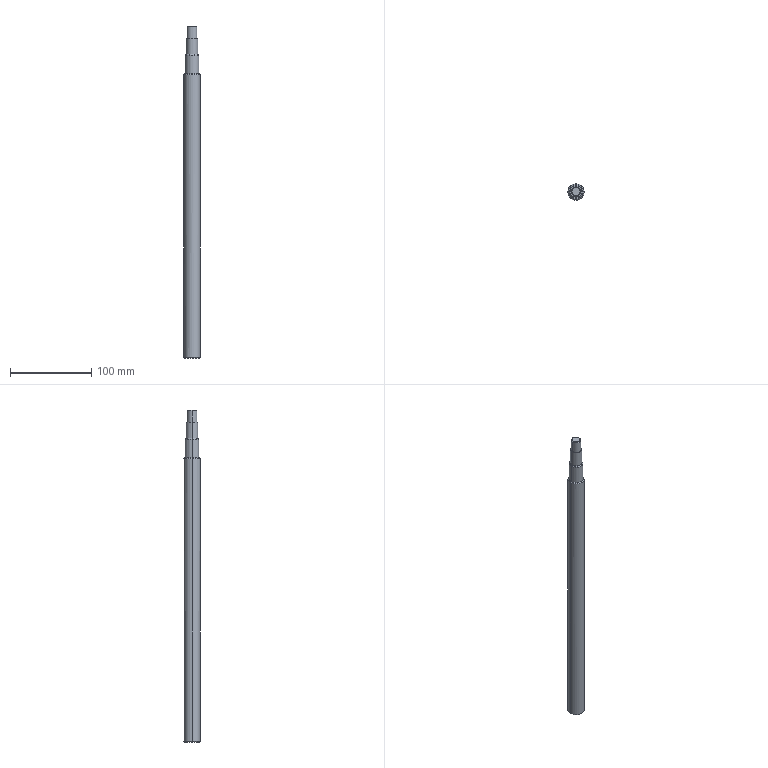Part | STEP file | fBY02F02M-00-27A | 1 solid | 21 faces | box 20 x 20 x 409 mm | volume 120074 mm3 | cylinder 8 | cone 8 | plane 5 | commonest cylinder face diameters 12 x2 14 x2 17 x2 20 x2
STEP:
#1=CARTESIAN_POINT('',(0.,0.,0.));
#2=DIRECTION('',(0.,0.,1.));
#3=DIRECTION('',(1.,0.,0.));
#4=AXIS2_PLACEMENT_3D('',#1,#2,#3);
#5=CARTESIAN_POINT('',(-10.,0.,349.));
#6=VERTEX_POINT('',#5);
#7=CARTESIAN_POINT('',(10.,0.,349.));
#8=VERTEX_POINT('',#7);
#9=CARTESIAN_POINT('',(0.,0.,349.));
#10=DIRECTION('',(0.,0.,-1.));
#11=DIRECTION('',(-1.,0.,0.));
#12=AXIS2_PLACEMENT_3D('',#9,#10,#11);
#13=CIRCLE('',#12,10.);
#14=CARTESIAN_POINT('',(0.,0.,350.));
#15=DIRECTION('',(0.,0.,-1.));
#16=DIRECTION('',(-1.,0.,0.));
#17=AXIS2_PLACEMENT_3D('',#14,#15,#16);
#18=CYLINDRICAL_SURFACE('',#17,10.);
#19=CARTESIAN_POINT('',(0.,1.));
#20=DIRECTION('',(1.,0.));
#21=VECTOR('',#20,1.);
#22=LINE('',#19,#21);
#23=(GEOMETRIC_REPRESENTATION_CONTEXT(2)PARAMETRIC_REPRESENTATION_CONTEXT()REPRESENTATION_CONTEXT('',''));
#24=DEFINITIONAL_REPRESENTATION('',(#22),#23);
#25=PCURVE('',#18,#24);
#26=CARTESIAN_POINT('',(0.,0.,349.));
#27=DIRECTION('',(0.,0.,-1.));
#28=DIRECTION('',(-1.,0.,0.));
#29=AXIS2_PLACEMENT_3D('',#26,#27,#28);
#30=CONICAL_SURFACE('',#29,10.,0.7854);
#31=CARTESIAN_POINT('',(0.,0.));
#32=DIRECTION('',(1.,0.));
#33=VECTOR('',#32,1.);
#34=LINE('',#31,#33);
#35=(GEOMETRIC_REPRESENTATION_CONTEXT(2)PARAMETRIC_REPRESENTATION_CONTEXT()REPRESENTATION_CONTEXT('',''));
#36=DEFINITIONAL_REPRESENTATION('',(#34),#35);
#37=PCURVE('',#30,#36);
#38=SURFACE_CURVE('',#13,(#25,#37),.PCURVE_S1.);
#39=EDGE_CURVE('',#6,#8,#38,.T.);
#40=ORIENTED_EDGE('',*,*,#39,.T.);
#41=CARTESIAN_POINT('',(10.,0.,1.));
#42=VERTEX_POINT('',#41);
#43=CARTESIAN_POINT('',(10.,0.,350.));
#44=DIRECTION('',(0.,0.,-1.));
#45=VECTOR('',#44,1.);
#46=LINE('',#43,#45);
#47=CARTESIAN_POINT('',(3.142,0.));
#48=DIRECTION('',(0.,1.));
#49=VECTOR('',#48,1.);
#50=LINE('',#47,#49);
#51=(GEOMETRIC_REPRESENTATION_CONTEXT(2)PARAMETRIC_REPRESENTATION_CONTEXT()REPRESENTATION_CONTEXT('',''));
#52=DEFINITIONAL_REPRESENTATION('',(#50),#51);
#53=PCURVE('',#18,#52);
#54=CARTESIAN_POINT('',(0.,0.,350.));
#55=DIRECTION('',(0.,0.,-1.));
#56=DIRECTION('',(-1.,0.,0.));
#57=AXIS2_PLACEMENT_3D('',#54,#55,#56);
#58=CYLINDRICAL_SURFACE('',#57,10.);
#59=CARTESIAN_POINT('',(3.142,0.));
#60=DIRECTION('',(0.,1.));
#61=VECTOR('',#60,1.);
#62=LINE('',#59,#61);
#63=(GEOMETRIC_REPRESENTATION_CONTEXT(2)PARAMETRIC_REPRESENTATION_CONTEXT()REPRESENTATION_CONTEXT('',''));
#64=DEFINITIONAL_REPRESENTATION('',(#62),#63);
#65=PCURVE('',#58,#64);
#66=SURFACE_CURVE('',#46,(#53,#65),.PCURVE_S1.);
#67=EDGE_CURVE('',#8,#42,#66,.T.);
#68=ORIENTED_EDGE('',*,*,#67,.T.);
#69=CARTESIAN_POINT('',(0.,10.,1.));
#70=VERTEX_POINT('',#69);
#71=CARTESIAN_POINT('',(0.,0.,1.));
#72=DIRECTION('',(0.,0.,1.));
#73=DIRECTION('',(-1.,0.,0.));
#74=AXIS2_PLACEMENT_3D('',#71,#72,#73);
#75=CIRCLE('',#74,10.);
#76=CARTESIAN_POINT('',(6.283,349.));
#77=DIRECTION('',(-1.,0.));
#78=VECTOR('',#77,1.);
#79=LINE('',#76,#78);
#80=(GEOMETRIC_REPRESENTATION_CONTEXT(2)PARAMETRIC_REPRESENTATION_CONTEXT()REPRESENTATION_CONTEXT('',''));
#81=DEFINITIONAL_REPRESENTATION('',(#79),#80);
#82=PCURVE('',#18,#81);
#83=CARTESIAN_POINT('',(0.,0.,1.));
#84=DIRECTION('',(0.,0.,1.));
#85=DIRECTION('',(0.,-1.,0.));
#86=AXIS2_PLACEMENT_3D('',#83,#84,#85);
#87=CONICAL_SURFACE('',#86,10.,0.7854);
#88=CARTESIAN_POINT('',(-1.571,0.));
#89=DIRECTION('',(1.,0.));
#90=VECTOR('',#89,1.);
#91=LINE('',#88,#90);
#92=(GEOMETRIC_REPRESENTATION_CONTEXT(2)PARAMETRIC_REPRESENTATION_CONTEXT()REPRESENTATION_CONTEXT('',''));
#93=DEFINITIONAL_REPRESENTATION('',(#91),#92);
#94=PCURVE('',#87,#93);
#95=SURFACE_CURVE('',#75,(#82,#94),.PCURVE_S1.);
#96=EDGE_CURVE('',#42,#70,#95,.T.);
#97=ORIENTED_EDGE('',*,*,#96,.T.);
#98=CARTESIAN_POINT('',(-10.,0.,1.));
#99=VERTEX_POINT('',#98);
#100=CARTESIAN_POINT('',(0.,0.,1.));
#101=DIRECTION('',(0.,0.,1.));
#102=DIRECTION('',(-1.,0.,0.));
#103=AXIS2_PLACEMENT_3D('',#100,#101,#102);
#104=CIRCLE('',#103,10.);
#105=CARTESIAN_POINT('',(6.283,349.));
#106=DIRECTION('',(-1.,0.));
#107=VECTOR('',#106,1.);
#108=LINE('',#105,#107);
#109=(GEOMETRIC_REPRESENTATION_CONTEXT(2)PARAMETRIC_REPRESENTATION_CONTEXT()REPRESENTATION_CONTEXT('',''));
#110=DEFINITIONAL_REPRESENTATION('',(#108),#109);
#111=PCURVE('',#18,#110);
#112=CARTESIAN_POINT('',(0.,0.,1.));
#113=DIRECTION('',(0.,0.,1.));
#114=DIRECTION('',(0.,-1.,0.));
#115=AXIS2_PLACEMENT_3D('',#112,#113,#114);
#116=CONICAL_SURFACE('',#115,10.,0.7854);
#117=CARTESIAN_POINT('',(-1.571,0.));
#118=DIRECTION('',(1.,0.));
#119=VECTOR('',#118,1.);
#120=LINE('',#117,#119);
#121=(GEOMETRIC_REPRESENTATION_CONTEXT(2)PARAMETRIC_REPRESENTATION_CONTEXT()REPRESENTATION_CONTEXT('',''));
#122=DEFINITIONAL_REPRESENTATION('',(#120),#121);
#123=PCURVE('',#116,#122);
#124=SURFACE_CURVE('',#104,(#111,#123),.PCURVE_S1.);
#125=EDGE_CURVE('',#70,#99,#124,.T.);
#126=ORIENTED_EDGE('',*,*,#125,.T.);
#127=CARTESIAN_POINT('',(-10.,0.,350.));
#128=DIRECTION('',(0.,0.,-1.));
#129=VECTOR('',#128,1.);
#130=LINE('',#127,#129);
#131=CARTESIAN_POINT('',(0.,0.));
#132=DIRECTION('',(0.,1.));
#133=VECTOR('',#132,1.);
#134=LINE('',#131,#133);
#135=(GEOMETRIC_REPRESENTATION_CONTEXT(2)PARAMETRIC_REPRESENTATION_CONTEXT()REPRESENTATION_CONTEXT('',''));
#136=DEFINITIONAL_REPRESENTATION('',(#134),#135);
#137=PCURVE('',#18,#136);
#138=CARTESIAN_POINT('',(6.283,0.));
#139=DIRECTION('',(0.,1.));
#140=VECTOR('',#139,1.);
#141=LINE('',#138,#140);
#142=(GEOMETRIC_REPRESENTATION_CONTEXT(2)PARAMETRIC_REPRESENTATION_CONTEXT()REPRESENTATION_CONTEXT('',''));
#143=DEFINITIONAL_REPRESENTATION('',(#141),#142);
#144=PCURVE('',#58,#143);
#145=SURFACE_CURVE('',#130,(#137,#144),.PCURVE_S1.);
#146=EDGE_CURVE('',#6,#99,#145,.T.);
#147=ORIENTED_EDGE('',*,*,#146,.F.);
#148=EDGE_LOOP('',(#40,#68,#97,#126,#147));
#149=FACE_BOUND('',#148,.T.);
#150=ADVANCED_FACE('',(#149),#18,.T.);
#151=CARTESIAN_POINT('',(0.,-9.,0.));
#152=VERTEX_POINT('',#151);
#153=CARTESIAN_POINT('',(0.,9.,0.));
#154=VERTEX_POINT('',#153);
#155=CARTESIAN_POINT('',(0.,0.,0.));
#156=DIRECTION('',(0.,0.,1.));
#157=DIRECTION('',(0.,-1.,0.));
#158=AXIS2_PLACEMENT_3D('',#155,#156,#157);
#159=CIRCLE('',#158,9.);
#160=CARTESIAN_POINT('',(0.,-1.));
#161=DIRECTION('',(1.,0.));
#162=VECTOR('',#161,1.);
#163=LINE('',#160,#162);
#164=(GEOMETRIC_REPRESENTATION_CONTEXT(2)PARAMETRIC_REPRESENTATION_CONTEXT()REPRESENTATION_CONTEXT('',''));
#165=DEFINITIONAL_REPRESENTATION('',(#163),#164);
#166=PCURVE('',#87,#165);
#167=CARTESIAN_POINT('',(0.,0.,0.));
#168=DIRECTION('',(0.,0.,1.));
#169=DIRECTION('',(1.,0.,0.));
#170=AXIS2_PLACEMENT_3D('',#167,#168,#169);
#171=PLANE('',#170);
#172=CARTESIAN_POINT('',(0.,0.));
#173=DIRECTION('',(0.,-1.));
#174=AXIS2_PLACEMENT_2D('',#172,#173);
#175=CIRCLE('',#174,9.);
#176=(GEOMETRIC_REPRESENTATION_CONTEXT(2)PARAMETRIC_REPRESENTATION_CONTEXT()REPRESENTATION_CONTEXT('',''));
#177=DEFINITIONAL_REPRESENTATION('',(#175),#176);
#178=PCURVE('',#171,#177);
#179=SURFACE_CURVE('',#159,(#166,#178),.PCURVE_S1.);
#180=EDGE_CURVE('',#152,#154,#179,.T.);
#181=ORIENTED_EDGE('',*,*,#180,.T.);
#182=CARTESIAN_POINT('',(0.,10.,1.));
#183=DIRECTION('',(0.,0.7071,0.7071));
#184=VECTOR('',#183,1.);
#185=LINE('',#182,#184);
#186=CARTESIAN_POINT('',(3.142,0.));
#187=DIRECTION('',(0.,1.));
#188=VECTOR('',#187,1.);
#189=LINE('',#186,#188);
#190=(GEOMETRIC_REPRESENTATION_CONTEXT(2)PARAMETRIC_REPRESENTATION_CONTEXT()REPRESENTATION_CONTEXT('',''));
#191=DEFINITIONAL_REPRESENTATION('',(#189),#190);
#192=PCURVE('',#87,#191);
#193=CARTESIAN_POINT('',(3.142,0.));
#194=DIRECTION('',(0.,1.));
#195=VECTOR('',#194,1.);
#196=LINE('',#193,#195);
#197=(GEOMETRIC_REPRESENTATION_CONTEXT(2)PARAMETRIC_REPRESENTATION_CONTEXT()REPRESENTATION_CONTEXT('',''));
#198=DEFINITIONAL_REPRESENTATION('',(#196),#197);
#199=PCURVE('',#116,#198);
#200=SURFACE_CURVE('',#185,(#192,#199),.PCURVE_S1.);
#201=EDGE_CURVE('',#154,#70,#200,.T.);
#202=ORIENTED_EDGE('',*,*,#201,.T.);
#203=ORIENTED_EDGE('',*,*,#96,.F.);
#204=CARTESIAN_POINT('',(0.,-10.,1.));
#205=VERTEX_POINT('',#204);
#206=CARTESIAN_POINT('',(0.,0.,1.));
#207=DIRECTION('',(0.,0.,1.));
#208=DIRECTION('',(-1.,0.,0.));
#209=AXIS2_PLACEMENT_3D('',#206,#207,#208);
#210=CIRCLE('',#209,10.);
#211=CARTESIAN_POINT('',(-1.571,0.));
#212=DIRECTION('',(1.,0.));
#213=VECTOR('',#212,1.);
#214=LINE('',#211,#213);
#215=(GEOMETRIC_REPRESENTATION_CONTEXT(2)PARAMETRIC_REPRESENTATION_CONTEXT()REPRESENTATION_CONTEXT('',''));
#216=DEFINITIONAL_REPRESENTATION('',(#214),#215);
#217=PCURVE('',#87,#216);
#218=CARTESIAN_POINT('',(6.283,349.));
#219=DIRECTION('',(-1.,0.));
#220=VECTOR('',#219,1.);
#221=LINE('',#218,#220);
#222=(GEOMETRIC_REPRESENTATION_CONTEXT(2)PARAMETRIC_REPRESENTATION_CONTEXT()REPRESENTATION_CONTEXT('',''));
#223=DEFINITIONAL_REPRESENTATION('',(#221),#222);
#224=PCURVE('',#58,#223);
#225=SURFACE_CURVE('',#210,(#217,#224),.PCURVE_S1.);
#226=EDGE_CURVE('',#205,#42,#225,.T.);
#227=ORIENTED_EDGE('',*,*,#226,.F.);
#228=CARTESIAN_POINT('',(0.,-10.,1.));
#229=DIRECTION('',(0.,-0.7071,0.7071));
#230=VECTOR('',#229,1.);
#231=LINE('',#228,#230);
#232=CARTESIAN_POINT('',(0.,0.));
#233=DIRECTION('',(0.,1.));
#234=VECTOR('',#233,1.);
#235=LINE('',#232,#234);
#236=(GEOMETRIC_REPRESENTATION_CONTEXT(2)PARAMETRIC_REPRESENTATION_CONTEXT()REPRESENTATION_CONTEXT('',''));
#237=DEFINITIONAL_REPRESENTATION('',(#235),#236);
#238=PCURVE('',#87,#237);
#239=CARTESIAN_POINT('',(6.283,0.));
#240=DIRECTION('',(0.,1.));
#241=VECTOR('',#240,1.);
#242=LINE('',#239,#241);
#243=(GEOMETRIC_REPRESENTATION_CONTEXT(2)PARAMETRIC_REPRESENTATION_CONTEXT()REPRESENTATION_CONTEXT('',''));
#244=DEFINITIONAL_REPRESENTATION('',(#242),#243);
#245=PCURVE('',#116,#244);
#246=SURFACE_CURVE('',#231,(#238,#245),.PCURVE_S1.);
#247=EDGE_CURVE('',#152,#205,#246,.T.);
#248=ORIENTED_EDGE('',*,*,#247,.F.);
#249=EDGE_LOOP('',(#181,#202,#203,#227,#248));
#250=FACE_BOUND('',#249,.T.);
#251=ADVANCED_FACE('',(#250),#87,.T.);
#252=CARTESIAN_POINT('',(-9.,0.,350.));
#253=VERTEX_POINT('',#252);
#254=CARTESIAN_POINT('',(9.,0.,350.));
#255=VERTEX_POINT('',#254);
#256=CARTESIAN_POINT('',(0.,0.,350.));
#257=DIRECTION('',(0.,0.,-1.));
#258=DIRECTION('',(-1.,0.,0.));
#259=AXIS2_PLACEMENT_3D('',#256,#257,#258);
#260=CIRCLE('',#259,9.);
#261=CARTESIAN_POINT('',(0.,-1.));
#262=DIRECTION('',(1.,0.));
#263=VECTOR('',#262,1.);
#264=LINE('',#261,#263);
#265=(GEOMETRIC_REPRESENTATION_CONTEXT(2)PARAMETRIC_REPRESENTATION_CONTEXT()REPRESENTATION_CONTEXT('',''));
#266=DEFINITIONAL_REPRESENTATION('',(#264),#265);
#267=PCURVE('',#30,#266);
#268=CARTESIAN_POINT('',(0.,0.,350.));
#269=DIRECTION('',(0.,0.,1.));
#270=DIRECTION('',(1.,0.,0.));
#271=AXIS2_PLACEMENT_3D('',#268,#269,#270);
#272=PLANE('',#271);
#273=CARTESIAN_POINT('',(-9.,0.));
#274=CARTESIAN_POINT('',(-9.,15.588));
#275=CARTESIAN_POINT('',(4.5,7.794));
#276=CARTESIAN_POINT('',(18.,0.));
#277=CARTESIAN_POINT('',(4.5,-7.794));
#278=CARTESIAN_POINT('',(-9.,-15.588));
#279=CARTESIAN_POINT('',(-9.,0.));
#280=(BOUNDED_CURVE()B_SPLINE_CURVE(2,(#273,#274,#275,#276,#277,#278,#279),.UNSPECIFIED.,.T.,.F.)B_SPLINE_CURVE_WITH_KNOTS((1,2,2,2,2,1),(-2.094,0.,2.094,4.189,6.283,8.378),.UNSPECIFIED.)CURVE()GEOMETRIC_REPRESENTATION_ITEM()RATIONAL_B_SPLINE_CURVE((1.,0.5,1.,0.5,1.,0.5,1.))REPRESENTATION_ITEM(''));
#281=(GEOMETRIC_REPRESENTATION_CONTEXT(2)PARAMETRIC_REPRESENTATION_CONTEXT()REPRESENTATION_CONTEXT('',''));
#282=DEFINITIONAL_REPRESENTATION('',(#280),#281);
#283=PCURVE('',#272,#282);
#284=SURFACE_CURVE('',#260,(#267,#283),.PCURVE_S1.);
#285=EDGE_CURVE('',#253,#255,#284,.T.);
#286=ORIENTED_EDGE('',*,*,#285,.T.);
#287=CARTESIAN_POINT('',(10.,0.,349.));
#288=DIRECTION('',(0.7071,0.,-0.7071));
#289=VECTOR('',#288,1.);
#290=LINE('',#287,#289);
#291=CARTESIAN_POINT('',(3.142,0.));
#292=DIRECTION('',(0.,1.));
#293=VECTOR('',#292,1.);
#294=LINE('',#291,#293);
#295=(GEOMETRIC_REPRESENTATION_CONTEXT(2)PARAMETRIC_REPRESENTATION_CONTEXT()REPRESENTATION_CONTEXT('',''));
#296=DEFINITIONAL_REPRESENTATION('',(#294),#295);
#297=PCURVE('',#30,#296);
#298=CARTESIAN_POINT('',(0.,0.,349.));
#299=DIRECTION('',(0.,0.,-1.));
#300=DIRECTION('',(-1.,0.,0.));
#301=AXIS2_PLACEMENT_3D('',#298,#299,#300);
#302=CONICAL_SURFACE('',#301,10.,0.7854);
#303=CARTESIAN_POINT('',(3.142,0.));
#304=DIRECTION('',(0.,1.));
#305=VECTOR('',#304,1.);
#306=LINE('',#303,#305);
#307=(GEOMETRIC_REPRESENTATION_CONTEXT(2)PARAMETRIC_REPRESENTATION_CONTEXT()REPRESENTATION_CONTEXT('',''));
#308=DEFINITIONAL_REPRESENTATION('',(#306),#307);
#309=PCURVE('',#302,#308);
#310=SURFACE_CURVE('',#290,(#297,#309),.PCURVE_S1.);
#311=EDGE_CURVE('',#255,#8,#310,.T.);
#312=ORIENTED_EDGE('',*,*,#311,.T.);
#313=ORIENTED_EDGE('',*,*,#39,.F.);
#314=CARTESIAN_POINT('',(-10.,0.,349.));
#315=DIRECTION('',(-0.7071,0.,-0.7071));
#316=VECTOR('',#315,1.);
#317=LINE('',#314,#316);
#318=CARTESIAN_POINT('',(0.,0.));
#319=DIRECTION('',(0.,1.));
#320=VECTOR('',#319,1.);
#321=LINE('',#318,#320);
#322=(GEOMETRIC_REPRESENTATION_CONTEXT(2)PARAMETRIC_REPRESENTATION_CONTEXT()REPRESENTATION_CONTEXT('',''));
#323=DEFINITIONAL_REPRESENTATION('',(#321),#322);
#324=PCURVE('',#30,#323);
#325=CARTESIAN_POINT('',(6.283,0.));
#326=DIRECTION('',(0.,1.));
#327=VECTOR('',#326,1.);
#328=LINE('',#325,#327);
#329=(GEOMETRIC_REPRESENTATION_CONTEXT(2)PARAMETRIC_REPRESENTATION_CONTEXT()REPRESENTATION_CONTEXT('',''));
#330=DEFINITIONAL_REPRESENTATION('',(#328),#329);
#331=PCURVE('',#302,#330);
#332=SURFACE_CURVE('',#317,(#324,#331),.PCURVE_S1.);
#333=EDGE_CURVE('',#253,#6,#332,.T.);
#334=ORIENTED_EDGE('',*,*,#333,.F.);
#335=EDGE_LOOP('',(#286,#312,#313,#334));
#336=FACE_BOUND('',#335,.T.);
#337=ADVANCED_FACE('',(#336),#30,.T.);
#338=CARTESIAN_POINT('',(-8.5,0.,373.));
#339=VERTEX_POINT('',#338);
#340=CARTESIAN_POINT('',(8.5,0.,373.));
#341=VERTEX_POINT('',#340);
#342=CARTESIAN_POINT('',(0.,0.,373.));
#343=DIRECTION('',(0.,0.,-1.));
#344=DIRECTION('',(-1.,0.,0.));
#345=AXIS2_PLACEMENT_3D('',#342,#343,#344);
#346=CIRCLE('',#345,8.5);
#347=CARTESIAN_POINT('',(0.,0.,374.));
#348=DIRECTION('',(0.,0.,-1.));
#349=DIRECTION('',(-1.,0.,0.));
#350=AXIS2_PLACEMENT_3D('',#347,#348,#349);
#351=CYLINDRICAL_SURFACE('',#350,8.5);
#352=CARTESIAN_POINT('',(0.,1.));
#353=DIRECTION('',(1.,0.));
#354=VECTOR('',#353,1.);
#355=LINE('',#352,#354);
#356=(GEOMETRIC_REPRESENTATION_CONTEXT(2)PARAMETRIC_REPRESENTATION_CONTEXT()REPRESENTATION_CONTEXT('',''));
#357=DEFINITIONAL_REPRESENTATION('',(#355),#356);
#358=PCURVE('',#351,#357);
#359=CARTESIAN_POINT('',(0.,0.,373.));
#360=DIRECTION('',(0.,0.,-1.));
#361=DIRECTION('',(-1.,0.,0.));
#362=AXIS2_PLACEMENT_3D('',#359,#360,#361);
#363=CONICAL_SURFACE('',#362,8.5,0.7854);
#364=CARTESIAN_POINT('',(0.,0.));
#365=DIRECTION('',(1.,0.));
#366=VECTOR('',#365,1.);
#367=LINE('',#364,#366);
#368=(GEOMETRIC_REPRESENTATION_CONTEXT(2)PARAMETRIC_REPRESENTATION_CONTEXT()REPRESENTATION_CONTEXT('',''));
#369=DEFINITIONAL_REPRESENTATION('',(#367),#368);
#370=PCURVE('',#363,#369);
#371=SURFACE_CURVE('',#346,(#358,#370),.PCURVE_S1.);
#372=EDGE_CURVE('',#339,#341,#371,.T.);
#373=ORIENTED_EDGE('',*,*,#372,.T.);
#374=CARTESIAN_POINT('',(8.5,0.,350.));
#375=VERTEX_POINT('',#374);
#376=CARTESIAN_POINT('',(8.5,0.,374.));
#377=DIRECTION('',(0.,0.,-1.));
#378=VECTOR('',#377,1.);
#379=LINE('',#376,#378);
#380=CARTESIAN_POINT('',(3.142,0.));
#381=DIRECTION('',(0.,1.));
#382=VECTOR('',#381,1.);
#383=LINE('',#380,#382);
#384=(GEOMETRIC_REPRESENTATION_CONTEXT(2)PARAMETRIC_REPRESENTATION_CONTEXT()REPRESENTATION_CONTEXT('',''));
#385=DEFINITIONAL_REPRESENTATION('',(#383),#384);
#386=PCURVE('',#351,#385);
#387=CARTESIAN_POINT('',(0.,0.,374.));
#388=DIRECTION('',(0.,0.,-1.));
#389=DIRECTION('',(-1.,0.,0.));
#390=AXIS2_PLACEMENT_3D('',#387,#388,#389);
#391=CYLINDRICAL_SURFACE('',#390,8.5);
#392=CARTESIAN_POINT('',(3.142,0.));
#393=DIRECTION('',(0.,1.));
#394=VECTOR('',#393,1.);
#395=LINE('',#392,#394);
#396=(GEOMETRIC_REPRESENTATION_CONTEXT(2)PARAMETRIC_REPRESENTATION_CONTEXT()REPRESENTATION_CONTEXT('',''));
#397=DEFINITIONAL_REPRESENTATION('',(#395),#396);
#398=PCURVE('',#391,#397);
#399=SURFACE_CURVE('',#379,(#386,#398),.PCURVE_S1.);
#400=EDGE_CURVE('',#341,#375,#399,.T.);
#401=ORIENTED_EDGE('',*,*,#400,.T.);
#402=CARTESIAN_POINT('',(-8.5,0.,350.));
#403=VERTEX_POINT('',#402);
#404=CARTESIAN_POINT('',(0.,0.,350.));
#405=DIRECTION('',(0.,0.,-1.));
#406=DIRECTION('',(-1.,0.,0.));
#407=AXIS2_PLACEMENT_3D('',#404,#405,#406);
#408=CIRCLE('',#407,8.5);
#409=CARTESIAN_POINT('',(0.,24.));
#410=DIRECTION('',(1.,0.));
#411=VECTOR('',#410,1.);
#412=LINE('',#409,#411);
#413=(GEOMETRIC_REPRESENTATION_CONTEXT(2)PARAMETRIC_REPRESENTATION_CONTEXT()REPRESENTATION_CONTEXT('',''));
#414=DEFINITIONAL_REPRESENTATION('',(#412),#413);
#415=PCURVE('',#351,#414);
#416=CARTESIAN_POINT('',(-8.5,0.));
#417=CARTESIAN_POINT('',(-8.5,14.722));
#418=CARTESIAN_POINT('',(4.25,7.361));
#419=CARTESIAN_POINT('',(17.,0.));
#420=CARTESIAN_POINT('',(4.25,-7.361));
#421=CARTESIAN_POINT('',(-8.5,-14.722));
#422=CARTESIAN_POINT('',(-8.5,0.));
#423=(BOUNDED_CURVE()B_SPLINE_CURVE(2,(#416,#417,#418,#419,#420,#421,#422),.UNSPECIFIED.,.T.,.F.)B_SPLINE_CURVE_WITH_KNOTS((1,2,2,2,2,1),(-2.094,0.,2.094,4.189,6.283,8.378),.UNSPECIFIED.)CURVE()GEOMETRIC_REPRESENTATION_ITEM()RATIONAL_B_SPLINE_CURVE((1.,0.5,1.,0.5,1.,0.5,1.))REPRESENTATION_ITEM(''));
#424=(GEOMETRIC_REPRESENTATION_CONTEXT(2)PARAMETRIC_REPRESENTATION_CONTEXT()REPRESENTATION_CONTEXT('',''));
#425=DEFINITIONAL_REPRESENTATION('',(#423),#424);
#426=PCURVE('',#272,#425);
#427=SURFACE_CURVE('',#408,(#415,#426),.PCURVE_S1.);
#428=EDGE_CURVE('',#403,#375,#427,.T.);
#429=ORIENTED_EDGE('',*,*,#428,.F.);
#430=CARTESIAN_POINT('',(-8.5,0.,374.));
#431=DIRECTION('',(0.,0.,-1.));
#432=VECTOR('',#431,1.);
#433=LINE('',#430,#432);
#434=CARTESIAN_POINT('',(0.,0.));
#435=DIRECTION('',(0.,1.));
#436=VECTOR('',#435,1.);
#437=LINE('',#434,#436);
#438=(GEOMETRIC_REPRESENTATION_CONTEXT(2)PARAMETRIC_REPRESENTATION_CONTEXT()REPRESENTATION_CONTEXT('',''));
#439=DEFINITIONAL_REPRESENTATION('',(#437),#438);
#440=PCURVE('',#351,#439);
#441=CARTESIAN_POINT('',(6.283,0.));
#442=DIRECTION('',(0.,1.));
#443=VECTOR('',#442,1.);
#444=LINE('',#441,#443);
#445=(GEOMETRIC_REPRESENTATION_CONTEXT(2)PARAMETRIC_REPRESENTATION_CONTEXT()REPRESENTATION_CONTEXT('',''));
#446=DEFINITIONAL_REPRESENTATION('',(#444),#445);
#447=PCURVE('',#391,#446);
#448=SURFACE_CURVE('',#433,(#440,#447),.PCURVE_S1.);
#449=EDGE_CURVE('',#339,#403,#448,.T.);
#450=ORIENTED_EDGE('',*,*,#449,.F.);
#451=EDGE_LOOP('',(#373,#401,#429,#450));
#452=FACE_BOUND('',#451,.T.);
#453=ADVANCED_FACE('',(#452),#351,.T.);
#454=CARTESIAN_POINT('',(-7.5,0.,374.));
#455=VERTEX_POINT('',#454);
#456=CARTESIAN_POINT('',(7.5,0.,374.));
#457=VERTEX_POINT('',#456);
#458=CARTESIAN_POINT('',(0.,0.,374.));
#459=DIRECTION('',(0.,0.,-1.));
#460=DIRECTION('',(-1.,0.,0.));
#461=AXIS2_PLACEMENT_3D('',#458,#459,#460);
#462=CIRCLE('',#461,7.5);
#463=CARTESIAN_POINT('',(0.,-1.));
#464=DIRECTION('',(1.,0.));
#465=VECTOR('',#464,1.);
#466=LINE('',#463,#465);
#467=(GEOMETRIC_REPRESENTATION_CONTEXT(2)PARAMETRIC_REPRESENTATION_CONTEXT()REPRESENTATION_CONTEXT('',''));
#468=DEFINITIONAL_REPRESENTATION('',(#466),#467);
#469=PCURVE('',#363,#468);
#470=CARTESIAN_POINT('',(0.,0.,374.));
#471=DIRECTION('',(0.,0.,1.));
#472=DIRECTION('',(1.,0.,0.));
#473=AXIS2_PLACEMENT_3D('',#470,#471,#472);
#474=PLANE('',#473);
#475=CARTESIAN_POINT('',(-7.5,0.));
#476=CARTESIAN_POINT('',(-7.5,12.99));
#477=CARTESIAN_POINT('',(3.75,6.495));
#478=CARTESIAN_POINT('',(15.,0.));
#479=CARTESIAN_POINT('',(3.75,-6.495));
#480=CARTESIAN_POINT('',(-7.5,-12.99));
#481=CARTESIAN_POINT('',(-7.5,0.));
#482=(BOUNDED_CURVE()B_SPLINE_CURVE(2,(#475,#476,#477,#478,#479,#480,#481),.UNSPECIFIED.,.T.,.F.)B_SPLINE_CURVE_WITH_KNOTS((1,2,2,2,2,1),(-2.094,0.,2.094,4.189,6.283,8.378),.UNSPECIFIED.)CURVE()GEOMETRIC_REPRESENTATION_ITEM()RATIONAL_B_SPLINE_CURVE((1.,0.5,1.,0.5,1.,0.5,1.))REPRESENTATION_ITEM(''));
#483=(GEOMETRIC_REPRESENTATION_CONTEXT(2)PARAMETRIC_REPRESENTATION_CONTEXT()REPRESENTATION_CONTEXT('',''));
#484=DEFINITIONAL_REPRESENTATION('',(#482),#483);
#485=PCURVE('',#474,#484);
#486=SURFACE_CURVE('',#462,(#469,#485),.PCURVE_S1.);
#487=EDGE_CURVE('',#455,#457,#486,.T.);
#488=ORIENTED_EDGE('',*,*,#487,.T.);
#489=CARTESIAN_POINT('',(8.5,0.,373.));
#490=DIRECTION('',(0.7071,0.,-0.7071));
#491=VECTOR('',#490,1.);
#492=LINE('',#489,#491);
#493=CARTESIAN_POINT('',(3.142,0.));
#494=DIRECTION('',(0.,1.));
#495=VECTOR('',#494,1.);
#496=LINE('',#493,#495);
#497=(GEOMETRIC_REPRESENTATION_CONTEXT(2)PARAMETRIC_REPRESENTATION_CONTEXT()REPRESENTATION_CONTEXT('',''));
#498=DEFINITIONAL_REPRESENTATION('',(#496),#497);
#499=PCURVE('',#363,#498);
#500=CARTESIAN_POINT('',(0.,0.,373.));
#501=DIRECTION('',(0.,0.,-1.));
#502=DIRECTION('',(-1.,0.,0.));
#503=AXIS2_PLACEMENT_3D('',#500,#501,#502);
#504=CONICAL_SURFACE('',#503,8.5,0.7854);
#505=CARTESIAN_POINT('',(3.142,0.));
#506=DIRECTION('',(0.,1.));
#507=VECTOR('',#506,1.);
#508=LINE('',#505,#507);
#509=(GEOMETRIC_REPRESENTATION_CONTEXT(2)PARAMETRIC_REPRESENTATION_CONTEXT()REPRESENTATION_CONTEXT('',''));
#510=DEFINITIONAL_REPRESENTATION('',(#508),#509);
#511=PCURVE('',#504,#510);
#512=SURFACE_CURVE('',#492,(#499,#511),.PCURVE_S1.);
#513=EDGE_CURVE('',#457,#341,#512,.T.);
#514=ORIENTED_EDGE('',*,*,#513,.T.);
#515=ORIENTED_EDGE('',*,*,#372,.F.);
#516=CARTESIAN_POINT('',(-8.5,0.,373.));
#517=DIRECTION('',(-0.7071,0.,-0.7071));
#518=VECTOR('',#517,1.);
#519=LINE('',#516,#518);
#520=CARTESIAN_POINT('',(0.,0.));
#521=DIRECTION('',(0.,1.));
#522=VECTOR('',#521,1.);
#523=LINE('',#520,#522);
#524=(GEOMETRIC_REPRESENTATION_CONTEXT(2)PARAMETRIC_REPRESENTATION_CONTEXT()REPRESENTATION_CONTEXT('',''));
#525=DEFINITIONAL_REPRESENTATION('',(#523),#524);
#526=PCURVE('',#363,#525);
#527=CARTESIAN_POINT('',(6.283,0.));
#528=DIRECTION('',(0.,1.));
#529=VECTOR('',#528,1.);
#530=LINE('',#527,#529);
#531=(GEOMETRIC_REPRESENTATION_CONTEXT(2)PARAMETRIC_REPRESENTATION_CONTEXT()REPRESENTATION_CONTEXT('',''));
#532=DEFINITIONAL_REPRESENTATION('',(#530),#531);
#533=PCURVE('',#504,#532);
#534=SURFACE_CURVE('',#519,(#526,#533),.PCURVE_S1.);
#535=EDGE_CURVE('',#455,#339,#534,.T.);
#536=ORIENTED_EDGE('',*,*,#535,.F.);
#537=EDGE_LOOP('',(#488,#514,#515,#536));
#538=FACE_BOUND('',#537,.T.);
#539=ADVANCED_FACE('',(#538),#363,.T.);
#540=CARTESIAN_POINT('',(-7.,0.,394.));
#541=VERTEX_POINT('',#540);
#542=CARTESIAN_POINT('',(7.,0.,394.));
#543=VERTEX_POINT('',#542);
#544=CARTESIAN_POINT('',(0.,0.,394.));
#545=DIRECTION('',(0.,0.,-1.));
#546=DIRECTION('',(-1.,0.,0.));
#547=AXIS2_PLACEMENT_3D('',#544,#545,#546);
#548=CIRCLE('',#547,7.);
#549=CARTESIAN_POINT('',(0.,0.,409.));
#550=DIRECTION('',(0.,0.,-1.));
#551=DIRECTION('',(-1.,0.,0.));
#552=AXIS2_PLACEMENT_3D('',#549,#550,#551);
#553=CYLINDRICAL_SURFACE('',#552,7.);
#554=CARTESIAN_POINT('',(0.,15.));
#555=DIRECTION('',(1.,0.));
#556=VECTOR('',#555,1.);
#557=LINE('',#554,#556);
#558=(GEOMETRIC_REPRESENTATION_CONTEXT(2)PARAMETRIC_REPRESENTATION_CONTEXT()REPRESENTATION_CONTEXT('',''));
#559=DEFINITIONAL_REPRESENTATION('',(#557),#558);
#560=PCURVE('',#553,#559);
#561=CARTESIAN_POINT('',(0.,0.,394.));
#562=DIRECTION('',(0.,0.,1.));
#563=DIRECTION('',(1.,0.,0.));
#564=AXIS2_PLACEMENT_3D('',#561,#562,#563);
#565=PLANE('',#564);
#566=CARTESIAN_POINT('',(-7.,0.));
#567=CARTESIAN_POINT('',(-7.,12.124));
#568=CARTESIAN_POINT('',(3.5,6.062));
#569=CARTESIAN_POINT('',(14.,0.));
#570=CARTESIAN_POINT('',(3.5,-6.062));
#571=CARTESIAN_POINT('',(-7.,-12.124));
#572=CARTESIAN_POINT('',(-7.,0.));
#573=(BOUNDED_CURVE()B_SPLINE_CURVE(2,(#566,#567,#568,#569,#570,#571,#572),.UNSPECIFIED.,.T.,.F.)B_SPLINE_CURVE_WITH_KNOTS((1,2,2,2,2,1),(-2.094,0.,2.094,4.189,6.283,8.378),.UNSPECIFIED.)CURVE()GEOMETRIC_REPRESENTATION_ITEM()RATIONAL_B_SPLINE_CURVE((1.,0.5,1.,0.5,1.,0.5,1.))REPRESENTATION_ITEM(''));
#574=(GEOMETRIC_REPRESENTATION_CONTEXT(2)PARAMETRIC_REPRESENTATION_CONTEXT()REPRESENTATION_CONTEXT('',''));
#575=DEFINITIONAL_REPRESENTATION('',(#573),#574);
#576=PCURVE('',#565,#575);
#577=SURFACE_CURVE('',#548,(#560,#576),.PCURVE_S1.);
#578=EDGE_CURVE('',#541,#543,#577,.T.);
#579=ORIENTED_EDGE('',*,*,#578,.T.);
#580=CARTESIAN_POINT('',(7.,0.,374.));
#581=VERTEX_POINT('',#580);
#582=CARTESIAN_POINT('',(7.,0.,409.));
#583=DIRECTION('',(0.,0.,-1.));
#584=VECTOR('',#583,1.);
#585=LINE('',#582,#584);
#586=CARTESIAN_POINT('',(3.142,0.));
#587=DIRECTION('',(0.,1.));
#588=VECTOR('',#587,1.);
#589=LINE('',#586,#588);
#590=(GEOMETRIC_REPRESENTATION_CONTEXT(2)PARAMETRIC_REPRESENTATION_CONTEXT()REPRESENTATION_CONTEXT('',''));
#591=DEFINITIONAL_REPRESENTATION('',(#589),#590);
#592=PCURVE('',#553,#591);
#593=CARTESIAN_POINT('',(0.,0.,409.));
#594=DIRECTION('',(0.,0.,-1.));
#595=DIRECTION('',(-1.,0.,0.));
#596=AXIS2_PLACEMENT_3D('',#593,#594,#595);
#597=CYLINDRICAL_SURFACE('',#596,7.);
#598=CARTESIAN_POINT('',(3.142,0.));
#599=DIRECTION('',(0.,1.));
#600=VECTOR('',#599,1.);
#601=LINE('',#598,#600);
#602=(GEOMETRIC_REPRESENTATION_CONTEXT(2)PARAMETRIC_REPRESENTATION_CONTEXT()REPRESENTATION_CONTEXT('',''));
#603=DEFINITIONAL_REPRESENTATION('',(#601),#602);
#604=PCURVE('',#597,#603);
#605=SURFACE_CURVE('',#585,(#592,#604),.PCURVE_S1.);
#606=EDGE_CURVE('',#543,#581,#605,.T.);
#607=ORIENTED_EDGE('',*,*,#606,.T.);
#608=CARTESIAN_POINT('',(-7.,0.,374.));
#609=VERTEX_POINT('',#608);
#610=CARTESIAN_POINT('',(0.,0.,374.));
#611=DIRECTION('',(0.,0.,-1.));
#612=DIRECTION('',(-1.,0.,0.));
#613=AXIS2_PLACEMENT_3D('',#610,#611,#612);
#614=CIRCLE('',#613,7.);
#615=CARTESIAN_POINT('',(0.,35.));
#616=DIRECTION('',(1.,0.));
#617=VECTOR('',#616,1.);
#618=LINE('',#615,#617);
#619=(GEOMETRIC_REPRESENTATION_CONTEXT(2)PARAMETRIC_REPRESENTATION_CONTEXT()REPRESENTATION_CONTEXT('',''));
#620=DEFINITIONAL_REPRESENTATION('',(#618),#619);
#621=PCURVE('',#553,#620);
#622=CARTESIAN_POINT('',(-7.,0.));
#623=CARTESIAN_POINT('',(-7.,12.124));
#624=CARTESIAN_POINT('',(3.5,6.062));
#625=CARTESIAN_POINT('',(14.,0.));
#626=CARTESIAN_POINT('',(3.5,-6.062));
#627=CARTESIAN_POINT('',(-7.,-12.124));
#628=CARTESIAN_POINT('',(-7.,0.));
#629=(BOUNDED_CURVE()B_SPLINE_CURVE(2,(#622,#623,#624,#625,#626,#627,#628),.UNSPECIFIED.,.T.,.F.)B_SPLINE_CURVE_WITH_KNOTS((1,2,2,2,2,1),(-2.094,0.,2.094,4.189,6.283,8.378),.UNSPECIFIED.)CURVE()GEOMETRIC_REPRESENTATION_ITEM()RATIONAL_B_SPLINE_CURVE((1.,0.5,1.,0.5,1.,0.5,1.))REPRESENTATION_ITEM(''));
#630=(GEOMETRIC_REPRESENTATION_CONTEXT(2)PARAMETRIC_REPRESENTATION_CONTEXT()REPRESENTATION_CONTEXT('',''));
#631=DEFINITIONAL_REPRESENTATION('',(#629),#630);
#632=PCURVE('',#474,#631);
#633=SURFACE_CURVE('',#614,(#621,#632),.PCURVE_S1.);
#634=EDGE_CURVE('',#609,#581,#633,.T.);
#635=ORIENTED_EDGE('',*,*,#634,.F.);
#636=CARTESIAN_POINT('',(-7.,0.,409.));
#637=DIRECTION('',(0.,0.,-1.));
#638=VECTOR('',#637,1.);
#639=LINE('',#636,#638);
#640=CARTESIAN_POINT('',(0.,0.));
#641=DIRECTION('',(0.,1.));
#642=VECTOR('',#641,1.);
#643=LINE('',#640,#642);
#644=(GEOMETRIC_REPRESENTATION_CONTEXT(2)PARAMETRIC_REPRESENTATION_CONTEXT()REPRESENTATION_CONTEXT('',''));
#645=DEFINITIONAL_REPRESENTATION('',(#643),#644);
#646=PCURVE('',#553,#645);
#647=CARTESIAN_POINT('',(6.283,0.));
#648=DIRECTION('',(0.,1.));
#649=VECTOR('',#648,1.);
#650=LINE('',#647,#649);
#651=(GEOMETRIC_REPRESENTATION_CONTEXT(2)PARAMETRIC_REPRESENTATION_CONTEXT()REPRESENTATION_CONTEXT('',''));
#652=DEFINITIONAL_REPRESENTATION('',(#650),#651);
#653=PCURVE('',#597,#652);
#654=SURFACE_CURVE('',#639,(#646,#653),.PCURVE_S1.);
#655=EDGE_CURVE('',#541,#609,#654,.T.);
#656=ORIENTED_EDGE('',*,*,#655,.F.);
#657=EDGE_LOOP('',(#579,#607,#635,#656));
#658=FACE_BOUND('',#657,.T.);
#659=ADVANCED_FACE('',(#658),#553,.T.);
#660=CARTESIAN_POINT('',(-6.,0.,394.));
#661=VERTEX_POINT('',#660);
#662=CARTESIAN_POINT('',(6.,0.,394.));
#663=VERTEX_POINT('',#662);
#664=CARTESIAN_POINT('',(0.,0.,394.));
#665=DIRECTION('',(0.,0.,-1.));
#666=DIRECTION('',(1.,0.,0.));
#667=AXIS2_PLACEMENT_3D('',#664,#665,#666);
#668=CIRCLE('',#667,6.);
#669=CARTESIAN_POINT('',(0.,0.,394.));
#670=DIRECTION('',(0.,0.,1.));
#671=DIRECTION('',(1.,0.,0.));
#672=AXIS2_PLACEMENT_3D('',#669,#670,#671);
#673=CYLINDRICAL_SURFACE('',#672,6.);
#674=CARTESIAN_POINT('',(6.283,0.));
#675=DIRECTION('',(-1.,0.));
#676=VECTOR('',#675,1.);
#677=LINE('',#674,#676);
#678=(GEOMETRIC_REPRESENTATION_CONTEXT(2)PARAMETRIC_REPRESENTATION_CONTEXT()REPRESENTATION_CONTEXT('',''));
#679=DEFINITIONAL_REPRESENTATION('',(#677),#678);
#680=PCURVE('',#673,#679);
#681=CARTESIAN_POINT('',(6.,0.));
#682=CARTESIAN_POINT('',(6.,-10.392));
#683=CARTESIAN_POINT('',(-3.,-5.196));
#684=CARTESIAN_POINT('',(-12.,0.));
#685=CARTESIAN_POINT('',(-3.,5.196));
#686=CARTESIAN_POINT('',(6.,10.392));
#687=CARTESIAN_POINT('',(6.,0.));
#688=(BOUNDED_CURVE()B_SPLINE_CURVE(2,(#681,#682,#683,#684,#685,#686,#687),.UNSPECIFIED.,.T.,.F.)B_SPLINE_CURVE_WITH_KNOTS((1,2,2,2,2,1),(-2.094,0.,2.094,4.189,6.283,8.378),.UNSPECIFIED.)CURVE()GEOMETRIC_REPRESENTATION_ITEM()RATIONAL_B_SPLINE_CURVE((1.,0.5,1.,0.5,1.,0.5,1.))REPRESENTATION_ITEM(''));
#689=(GEOMETRIC_REPRESENTATION_CONTEXT(2)PARAMETRIC_REPRESENTATION_CONTEXT()REPRESENTATION_CONTEXT('',''));
#690=DEFINITIONAL_REPRESENTATION('',(#688),#689);
#691=PCURVE('',#565,#690);
#692=SURFACE_CURVE('',#668,(#680,#691),.PCURVE_S1.);
#693=EDGE_CURVE('',#661,#663,#692,.T.);
#694=ORIENTED_EDGE('',*,*,#693,.F.);
#695=CARTESIAN_POINT('',(-6.,0.,408.));
#696=VERTEX_POINT('',#695);
#697=CARTESIAN_POINT('',(-6.,0.,394.));
#698=DIRECTION('',(0.,0.,1.));
#699=VECTOR('',#698,1.);
#700=LINE('',#697,#699);
#701=CARTESIAN_POINT('',(3.142,0.));
#702=DIRECTION('',(0.,1.));
#703=VECTOR('',#702,1.);
#704=LINE('',#701,#703);
#705=(GEOMETRIC_REPRESENTATION_CONTEXT(2)PARAMETRIC_REPRESENTATION_CONTEXT()REPRESENTATION_CONTEXT('',''));
#706=DEFINITIONAL_REPRESENTATION('',(#704),#705);
#707=PCURVE('',#673,#706);
#708=CARTESIAN_POINT('',(0.,0.,394.));
#709=DIRECTION('',(0.,0.,1.));
#710=DIRECTION('',(1.,0.,0.));
#711=AXIS2_PLACEMENT_3D('',#708,#709,#710);
#712=CYLINDRICAL_SURFACE('',#711,6.);
#713=CARTESIAN_POINT('',(3.142,0.));
#714=DIRECTION('',(0.,1.));
#715=VECTOR('',#714,1.);
#716=LINE('',#713,#715);
#717=(GEOMETRIC_REPRESENTATION_CONTEXT(2)PARAMETRIC_REPRESENTATION_CONTEXT()REPRESENTATION_CONTEXT('',''));
#718=DEFINITIONAL_REPRESENTATION('',(#716),#717);
#719=PCURVE('',#712,#718);
#720=SURFACE_CURVE('',#700,(#707,#719),.PCURVE_S1.);
#721=EDGE_CURVE('',#661,#696,#720,.T.);
#722=ORIENTED_EDGE('',*,*,#721,.T.);
#723=CARTESIAN_POINT('',(6.,0.,408.));
#724=VERTEX_POINT('',#723);
#725=CARTESIAN_POINT('',(0.,0.,408.));
#726=DIRECTION('',(0.,0.,-1.));
#727=DIRECTION('',(1.,0.,0.));
#728=AXIS2_PLACEMENT_3D('',#725,#726,#727);
#729=CIRCLE('',#728,6.);
#730=CARTESIAN_POINT('',(6.283,14.));
#731=DIRECTION('',(-1.,0.));
#732=VECTOR('',#731,1.);
#733=LINE('',#730,#732);
#734=(GEOMETRIC_REPRESENTATION_CONTEXT(2)PARAMETRIC_REPRESENTATION_CONTEXT()REPRESENTATION_CONTEXT('',''));
#735=DEFINITIONAL_REPRESENTATION('',(#733),#734);
#736=PCURVE('',#673,#735);
#737=CARTESIAN_POINT('',(0.,0.,408.));
#738=DIRECTION('',(0.,0.,-1.));
#739=DIRECTION('',(-1.,0.,0.));
#740=AXIS2_PLACEMENT_3D('',#737,#738,#739);
#741=CONICAL_SURFACE('',#740,6.,0.7854);
#742=CARTESIAN_POINT('',(-3.142,0.));
#743=DIRECTION('',(1.,0.));
#744=VECTOR('',#743,1.);
#745=LINE('',#742,#744);
#746=(GEOMETRIC_REPRESENTATION_CONTEXT(2)PARAMETRIC_REPRESENTATION_CONTEXT()REPRESENTATION_CONTEXT('',''));
#747=DEFINITIONAL_REPRESENTATION('',(#745),#746);
#748=PCURVE('',#741,#747);
#749=SURFACE_CURVE('',#729,(#736,#748),.PCURVE_S1.);
#750=EDGE_CURVE('',#696,#724,#749,.T.);
#751=ORIENTED_EDGE('',*,*,#750,.T.);
#752=CARTESIAN_POINT('',(6.,0.,394.));
#753=DIRECTION('',(0.,0.,1.));
#754=VECTOR('',#753,1.);
#755=LINE('',#752,#754);
#756=CARTESIAN_POINT('',(0.,0.));
#757=DIRECTION('',(0.,1.));
#758=VECTOR('',#757,1.);
#759=LINE('',#756,#758);
#760=(GEOMETRIC_REPRESENTATION_CONTEXT(2)PARAMETRIC_REPRESENTATION_CONTEXT()REPRESENTATION_CONTEXT('',''));
#761=DEFINITIONAL_REPRESENTATION('',(#759),#760);
#762=PCURVE('',#673,#761);
#763=CARTESIAN_POINT('',(6.283,0.));
#764=DIRECTION('',(0.,1.));
#765=VECTOR('',#764,1.);
#766=LINE('',#763,#765);
#767=(GEOMETRIC_REPRESENTATION_CONTEXT(2)PARAMETRIC_REPRESENTATION_CONTEXT()REPRESENTATION_CONTEXT('',''));
#768=DEFINITIONAL_REPRESENTATION('',(#766),#767);
#769=PCURVE('',#712,#768);
#770=SURFACE_CURVE('',#755,(#762,#769),.PCURVE_S1.);
#771=EDGE_CURVE('',#663,#724,#770,.T.);
#772=ORIENTED_EDGE('',*,*,#771,.F.);
#773=EDGE_LOOP('',(#694,#722,#751,#772));
#774=FACE_BOUND('',#773,.T.);
#775=ADVANCED_FACE('',(#774),#673,.T.);
#776=CARTESIAN_POINT('',(-5.,0.,409.));
#777=VERTEX_POINT('',#776);
#778=CARTESIAN_POINT('',(5.,0.,409.));
#779=VERTEX_POINT('',#778);
#780=CARTESIAN_POINT('',(0.,0.,409.));
#781=DIRECTION('',(0.,0.,-1.));
#782=DIRECTION('',(-1.,0.,0.));
#783=AXIS2_PLACEMENT_3D('',#780,#781,#782);
#784=CIRCLE('',#783,5.);
#785=CARTESIAN_POINT('',(0.,-1.));
#786=DIRECTION('',(1.,0.));
#787=VECTOR('',#786,1.);
#788=LINE('',#785,#787);
#789=(GEOMETRIC_REPRESENTATION_CONTEXT(2)PARAMETRIC_REPRESENTATION_CONTEXT()REPRESENTATION_CONTEXT('',''));
#790=DEFINITIONAL_REPRESENTATION('',(#788),#789);
#791=PCURVE('',#741,#790);
#792=CARTESIAN_POINT('',(0.,0.,409.));
#793=DIRECTION('',(0.,0.,1.));
#794=DIRECTION('',(1.,0.,0.));
#795=AXIS2_PLACEMENT_3D('',#792,#793,#794);
#796=PLANE('',#795);
#797=CARTESIAN_POINT('',(-5.,0.));
#798=CARTESIAN_POINT('',(-5.,8.66));
#799=CARTESIAN_POINT('',(2.5,4.33));
#800=CARTESIAN_POINT('',(10.,0.));
#801=CARTESIAN_POINT('',(2.5,-4.33));
#802=CARTESIAN_POINT('',(-5.,-8.66));
#803=CARTESIAN_POINT('',(-5.,0.));
#804=(BOUNDED_CURVE()B_SPLINE_CURVE(2,(#797,#798,#799,#800,#801,#802,#803),.UNSPECIFIED.,.T.,.F.)B_SPLINE_CURVE_WITH_KNOTS((1,2,2,2,2,1),(-2.094,0.,2.094,4.189,6.283,8.378),.UNSPECIFIED.)CURVE()GEOMETRIC_REPRESENTATION_ITEM()RATIONAL_B_SPLINE_CURVE((1.,0.5,1.,0.5,1.,0.5,1.))REPRESENTATION_ITEM(''));
#805=(GEOMETRIC_REPRESENTATION_CONTEXT(2)PARAMETRIC_REPRESENTATION_CONTEXT()REPRESENTATION_CONTEXT('',''));
#806=DEFINITIONAL_REPRESENTATION('',(#804),#805);
#807=PCURVE('',#796,#806);
#808=SURFACE_CURVE('',#784,(#791,#807),.PCURVE_S1.);
#809=EDGE_CURVE('',#777,#779,#808,.T.);
#810=ORIENTED_EDGE('',*,*,#809,.T.);
#811=CARTESIAN_POINT('',(6.,0.,408.));
#812=DIRECTION('',(0.7071,0.,-0.7071));
#813=VECTOR('',#812,1.);
#814=LINE('',#811,#813);
#815=CARTESIAN_POINT('',(3.142,0.));
#816=DIRECTION('',(0.,1.));
#817=VECTOR('',#816,1.);
#818=LINE('',#815,#817);
#819=(GEOMETRIC_REPRESENTATION_CONTEXT(2)PARAMETRIC_REPRESENTATION_CONTEXT()REPRESENTATION_CONTEXT('',''));
#820=DEFINITIONAL_REPRESENTATION('',(#818),#819);
#821=PCURVE('',#741,#820);
#822=CARTESIAN_POINT('',(0.,0.,408.));
#823=DIRECTION('',(0.,0.,-1.));
#824=DIRECTION('',(-1.,0.,0.));
#825=AXIS2_PLACEMENT_3D('',#822,#823,#824);
#826=CONICAL_SURFACE('',#825,6.,0.7854);
#827=CARTESIAN_POINT('',(3.142,0.));
#828=DIRECTION('',(0.,1.));
#829=VECTOR('',#828,1.);
#830=LINE('',#827,#829);
#831=(GEOMETRIC_REPRESENTATION_CONTEXT(2)PARAMETRIC_REPRESENTATION_CONTEXT()REPRESENTATION_CONTEXT('',''));
#832=DEFINITIONAL_REPRESENTATION('',(#830),#831);
#833=PCURVE('',#826,#832);
#834=SURFACE_CURVE('',#814,(#821,#833),.PCURVE_S1.);
#835=EDGE_CURVE('',#779,#724,#834,.T.);
#836=ORIENTED_EDGE('',*,*,#835,.T.);
#837=ORIENTED_EDGE('',*,*,#750,.F.);
#838=CARTESIAN_POINT('',(-6.,0.,408.));
#839=DIRECTION('',(-0.7071,0.,-0.7071));
#840=VECTOR('',#839,1.);
#841=LINE('',#838,#840);
#842=CARTESIAN_POINT('',(0.,0.));
#843=DIRECTION('',(0.,1.));
#844=VECTOR('',#843,1.);
#845=LINE('',#842,#844);
#846=(GEOMETRIC_REPRESENTATION_CONTEXT(2)PARAMETRIC_REPRESENTATION_CONTEXT()REPRESENTATION_CONTEXT('',''));
#847=DEFINITIONAL_REPRESENTATION('',(#845),#846);
#848=PCURVE('',#741,#847);
#849=CARTESIAN_POINT('',(6.283,0.));
#850=DIRECTION('',(0.,1.));
#851=VECTOR('',#850,1.);
#852=LINE('',#849,#851);
#853=(GEOMETRIC_REPRESENTATION_CONTEXT(2)PARAMETRIC_REPRESENTATION_CONTEXT()REPRESENTATION_CONTEXT('',''));
#854=DEFINITIONAL_REPRESENTATION('',(#852),#853);
#855=PCURVE('',#826,#854);
#856=SURFACE_CURVE('',#841,(#848,#855),.PCURVE_S1.);
#857=EDGE_CURVE('',#777,#696,#856,.T.);
#858=ORIENTED_EDGE('',*,*,#857,.F.);
#859=EDGE_LOOP('',(#810,#836,#837,#858));
#860=FACE_BOUND('',#859,.T.);
#861=ADVANCED_FACE('',(#860),#741,.T.);
#862=ORIENTED_EDGE('',*,*,#67,.F.);
#863=CARTESIAN_POINT('',(0.,0.,349.));
#864=DIRECTION('',(0.,0.,-1.));
#865=DIRECTION('',(-1.,0.,0.));
#866=AXIS2_PLACEMENT_3D('',#863,#864,#865);
#867=CIRCLE('',#866,10.);
#868=CARTESIAN_POINT('',(0.,1.));
#869=DIRECTION('',(1.,0.));
#870=VECTOR('',#869,1.);
#871=LINE('',#868,#870);
#872=(GEOMETRIC_REPRESENTATION_CONTEXT(2)PARAMETRIC_REPRESENTATION_CONTEXT()REPRESENTATION_CONTEXT('',''));
#873=DEFINITIONAL_REPRESENTATION('',(#871),#872);
#874=PCURVE('',#58,#873);
#875=CARTESIAN_POINT('',(0.,0.));
#876=DIRECTION('',(1.,0.));
#877=VECTOR('',#876,1.);
#878=LINE('',#875,#877);
#879=(GEOMETRIC_REPRESENTATION_CONTEXT(2)PARAMETRIC_REPRESENTATION_CONTEXT()REPRESENTATION_CONTEXT('',''));
#880=DEFINITIONAL_REPRESENTATION('',(#878),#879);
#881=PCURVE('',#302,#880);
#882=SURFACE_CURVE('',#867,(#874,#881),.PCURVE_S1.);
#883=EDGE_CURVE('',#8,#6,#882,.T.);
#884=ORIENTED_EDGE('',*,*,#883,.T.);
#885=ORIENTED_EDGE('',*,*,#146,.T.);
#886=CARTESIAN_POINT('',(0.,0.,1.));
#887=DIRECTION('',(0.,0.,1.));
#888=DIRECTION('',(-1.,0.,0.));
#889=AXIS2_PLACEMENT_3D('',#886,#887,#888);
#890=CIRCLE('',#889,10.);
#891=CARTESIAN_POINT('',(6.283,349.));
#892=DIRECTION('',(-1.,0.));
#893=VECTOR('',#892,1.);
#894=LINE('',#891,#893);
#895=(GEOMETRIC_REPRESENTATION_CONTEXT(2)PARAMETRIC_REPRESENTATION_CONTEXT()REPRESENTATION_CONTEXT('',''));
#896=DEFINITIONAL_REPRESENTATION('',(#894),#895);
#897=PCURVE('',#58,#896);
#898=CARTESIAN_POINT('',(4.712,0.));
#899=DIRECTION('',(1.,0.));
#900=VECTOR('',#899,1.);
#901=LINE('',#898,#900);
#902=(GEOMETRIC_REPRESENTATION_CONTEXT(2)PARAMETRIC_REPRESENTATION_CONTEXT()REPRESENTATION_CONTEXT('',''));
#903=DEFINITIONAL_REPRESENTATION('',(#901),#902);
#904=PCURVE('',#116,#903);
#905=SURFACE_CURVE('',#890,(#897,#904),.PCURVE_S1.);
#906=EDGE_CURVE('',#99,#205,#905,.T.);
#907=ORIENTED_EDGE('',*,*,#906,.T.);
#908=ORIENTED_EDGE('',*,*,#226,.T.);
#909=EDGE_LOOP('',(#862,#884,#885,#907,#908));
#910=FACE_BOUND('',#909,.T.);
#911=ADVANCED_FACE('',(#910),#58,.T.);
#912=ORIENTED_EDGE('',*,*,#201,.F.);
#913=CARTESIAN_POINT('',(0.,0.,0.));
#914=DIRECTION('',(0.,0.,1.));
#915=DIRECTION('',(0.,-1.,0.));
#916=AXIS2_PLACEMENT_3D('',#913,#914,#915);
#917=CIRCLE('',#916,9.);
#918=CARTESIAN_POINT('',(0.,-1.));
#919=DIRECTION('',(1.,0.));
#920=VECTOR('',#919,1.);
#921=LINE('',#918,#920);
#922=(GEOMETRIC_REPRESENTATION_CONTEXT(2)PARAMETRIC_REPRESENTATION_CONTEXT()REPRESENTATION_CONTEXT('',''));
#923=DEFINITIONAL_REPRESENTATION('',(#921),#922);
#924=PCURVE('',#116,#923);
#925=CARTESIAN_POINT('',(0.,0.));
#926=DIRECTION('',(0.,-1.));
#927=AXIS2_PLACEMENT_2D('',#925,#926);
#928=CIRCLE('',#927,9.);
#929=(GEOMETRIC_REPRESENTATION_CONTEXT(2)PARAMETRIC_REPRESENTATION_CONTEXT()REPRESENTATION_CONTEXT('',''));
#930=DEFINITIONAL_REPRESENTATION('',(#928),#929);
#931=PCURVE('',#171,#930);
#932=SURFACE_CURVE('',#917,(#924,#931),.PCURVE_S1.);
#933=EDGE_CURVE('',#154,#152,#932,.T.);
#934=ORIENTED_EDGE('',*,*,#933,.T.);
#935=ORIENTED_EDGE('',*,*,#247,.T.);
#936=ORIENTED_EDGE('',*,*,#906,.F.);
#937=ORIENTED_EDGE('',*,*,#125,.F.);
#938=EDGE_LOOP('',(#912,#934,#935,#936,#937));
#939=FACE_BOUND('',#938,.T.);
#940=ADVANCED_FACE('',(#939),#116,.T.);
#941=ORIENTED_EDGE('',*,*,#311,.F.);
#942=CARTESIAN_POINT('',(0.,0.,350.));
#943=DIRECTION('',(0.,0.,-1.));
#944=DIRECTION('',(-1.,0.,0.));
#945=AXIS2_PLACEMENT_3D('',#942,#943,#944);
#946=CIRCLE('',#945,9.);
#947=CARTESIAN_POINT('',(0.,-1.));
#948=DIRECTION('',(1.,0.));
#949=VECTOR('',#948,1.);
#950=LINE('',#947,#949);
#951=(GEOMETRIC_REPRESENTATION_CONTEXT(2)PARAMETRIC_REPRESENTATION_CONTEXT()REPRESENTATION_CONTEXT('',''));
#952=DEFINITIONAL_REPRESENTATION('',(#950),#951);
#953=PCURVE('',#302,#952);
#954=CARTESIAN_POINT('',(-9.,0.));
#955=CARTESIAN_POINT('',(-9.,15.588));
#956=CARTESIAN_POINT('',(4.5,7.794));
#957=CARTESIAN_POINT('',(18.,0.));
#958=CARTESIAN_POINT('',(4.5,-7.794));
#959=CARTESIAN_POINT('',(-9.,-15.588));
#960=CARTESIAN_POINT('',(-9.,0.));
#961=(BOUNDED_CURVE()B_SPLINE_CURVE(2,(#954,#955,#956,#957,#958,#959,#960),.UNSPECIFIED.,.T.,.F.)B_SPLINE_CURVE_WITH_KNOTS((1,2,2,2,2,1),(-2.094,0.,2.094,4.189,6.283,8.378),.UNSPECIFIED.)CURVE()GEOMETRIC_REPRESENTATION_ITEM()RATIONAL_B_SPLINE_CURVE((1.,0.5,1.,0.5,1.,0.5,1.))REPRESENTATION_ITEM(''));
#962=(GEOMETRIC_REPRESENTATION_CONTEXT(2)PARAMETRIC_REPRESENTATION_CONTEXT()REPRESENTATION_CONTEXT('',''));
#963=DEFINITIONAL_REPRESENTATION('',(#961),#962);
#964=PCURVE('',#272,#963);
#965=SURFACE_CURVE('',#946,(#953,#964),.PCURVE_S1.);
#966=EDGE_CURVE('',#255,#253,#965,.T.);
#967=ORIENTED_EDGE('',*,*,#966,.T.);
#968=ORIENTED_EDGE('',*,*,#333,.T.);
#969=ORIENTED_EDGE('',*,*,#883,.F.);
#970=EDGE_LOOP('',(#941,#967,#968,#969));
#971=FACE_BOUND('',#970,.T.);
#972=ADVANCED_FACE('',(#971),#302,.T.);
#973=ORIENTED_EDGE('',*,*,#180,.F.);
#974=ORIENTED_EDGE('',*,*,#933,.F.);
#975=EDGE_LOOP('',(#973,#974));
#976=FACE_BOUND('',#975,.T.);
#977=ADVANCED_FACE('',(#976),#171,.F.);
#978=ORIENTED_EDGE('',*,*,#428,.T.);
#979=CARTESIAN_POINT('',(0.,0.,350.));
#980=DIRECTION('',(0.,0.,-1.));
#981=DIRECTION('',(-1.,0.,0.));
#982=AXIS2_PLACEMENT_3D('',#979,#980,#981);
#983=CIRCLE('',#982,8.5);
#984=CARTESIAN_POINT('',(-8.5,0.));
#985=CARTESIAN_POINT('',(-8.5,14.722));
#986=CARTESIAN_POINT('',(4.25,7.361));
#987=CARTESIAN_POINT('',(17.,0.));
#988=CARTESIAN_POINT('',(4.25,-7.361));
#989=CARTESIAN_POINT('',(-8.5,-14.722));
#990=CARTESIAN_POINT('',(-8.5,0.));
#991=(BOUNDED_CURVE()B_SPLINE_CURVE(2,(#984,#985,#986,#987,#988,#989,#990),.UNSPECIFIED.,.T.,.F.)B_SPLINE_CURVE_WITH_KNOTS((1,2,2,2,2,1),(-2.094,0.,2.094,4.189,6.283,8.378),.UNSPECIFIED.)CURVE()GEOMETRIC_REPRESENTATION_ITEM()RATIONAL_B_SPLINE_CURVE((1.,0.5,1.,0.5,1.,0.5,1.))REPRESENTATION_ITEM(''));
#992=(GEOMETRIC_REPRESENTATION_CONTEXT(2)PARAMETRIC_REPRESENTATION_CONTEXT()REPRESENTATION_CONTEXT('',''));
#993=DEFINITIONAL_REPRESENTATION('',(#991),#992);
#994=PCURVE('',#272,#993);
#995=CARTESIAN_POINT('',(0.,24.));
#996=DIRECTION('',(1.,0.));
#997=VECTOR('',#996,1.);
#998=LINE('',#995,#997);
#999=(GEOMETRIC_REPRESENTATION_CONTEXT(2)PARAMETRIC_REPRESENTATION_CONTEXT()REPRESENTATION_CONTEXT('',''));
#1000=DEFINITIONAL_REPRESENTATION('',(#998),#999);
#1001=PCURVE('',#391,#1000);
#1002=SURFACE_CURVE('',#983,(#994,#1001),.PCURVE_S1.);
#1003=EDGE_CURVE('',#375,#403,#1002,.T.);
#1004=ORIENTED_EDGE('',*,*,#1003,.T.);
#1005=EDGE_LOOP('',(#978,#1004));
#1006=FACE_BOUND('',#1005,.T.);
#1007=ORIENTED_EDGE('',*,*,#285,.F.);
#1008=ORIENTED_EDGE('',*,*,#966,.F.);
#1009=EDGE_LOOP('',(#1007,#1008));
#1010=FACE_BOUND('',#1009,.T.);
#1011=ADVANCED_FACE('',(#1006,#1010),#272,.T.);
#1012=ORIENTED_EDGE('',*,*,#400,.F.);
#1013=CARTESIAN_POINT('',(0.,0.,373.));
#1014=DIRECTION('',(0.,0.,-1.));
#1015=DIRECTION('',(-1.,0.,0.));
#1016=AXIS2_PLACEMENT_3D('',#1013,#1014,#1015);
#1017=CIRCLE('',#1016,8.5);
#1018=CARTESIAN_POINT('',(0.,1.));
#1019=DIRECTION('',(1.,0.));
#1020=VECTOR('',#1019,1.);
#1021=LINE('',#1018,#1020);
#1022=(GEOMETRIC_REPRESENTATION_CONTEXT(2)PARAMETRIC_REPRESENTATION_CONTEXT()REPRESENTATION_CONTEXT('',''));
#1023=DEFINITIONAL_REPRESENTATION('',(#1021),#1022);
#1024=PCURVE('',#391,#1023);
#1025=CARTESIAN_POINT('',(0.,0.));
#1026=DIRECTION('',(1.,0.));
#1027=VECTOR('',#1026,1.);
#1028=LINE('',#1025,#1027);
#1029=(GEOMETRIC_REPRESENTATION_CONTEXT(2)PARAMETRIC_REPRESENTATION_CONTEXT()REPRESENTATION_CONTEXT('',''));
#1030=DEFINITIONAL_REPRESENTATION('',(#1028),#1029);
#1031=PCURVE('',#504,#1030);
#1032=SURFACE_CURVE('',#1017,(#1024,#1031),.PCURVE_S1.);
#1033=EDGE_CURVE('',#341,#339,#1032,.T.);
#1034=ORIENTED_EDGE('',*,*,#1033,.T.);
#1035=ORIENTED_EDGE('',*,*,#449,.T.);
#1036=ORIENTED_EDGE('',*,*,#1003,.F.);
#1037=EDGE_LOOP('',(#1012,#1034,#1035,#1036));
#1038=FACE_BOUND('',#1037,.T.);
#1039=ADVANCED_FACE('',(#1038),#391,.T.);
#1040=ORIENTED_EDGE('',*,*,#513,.F.);
#1041=CARTESIAN_POINT('',(0.,0.,374.));
#1042=DIRECTION('',(0.,0.,-1.));
#1043=DIRECTION('',(-1.,0.,0.));
#1044=AXIS2_PLACEMENT_3D('',#1041,#1042,#1043);
#1045=CIRCLE('',#1044,7.5);
#1046=CARTESIAN_POINT('',(0.,-1.));
#1047=DIRECTION('',(1.,0.));
#1048=VECTOR('',#1047,1.);
#1049=LINE('',#1046,#1048);
#1050=(GEOMETRIC_REPRESENTATION_CONTEXT(2)PARAMETRIC_REPRESENTATION_CONTEXT()REPRESENTATION_CONTEXT('',''));
#1051=DEFINITIONAL_REPRESENTATION('',(#1049),#1050);
#1052=PCURVE('',#504,#1051);
#1053=CARTESIAN_POINT('',(-7.5,0.));
#1054=CARTESIAN_POINT('',(-7.5,12.99));
#1055=CARTESIAN_POINT('',(3.75,6.495));
#1056=CARTESIAN_POINT('',(15.,0.));
#1057=CARTESIAN_POINT('',(3.75,-6.495));
#1058=CARTESIAN_POINT('',(-7.5,-12.99));
#1059=CARTESIAN_POINT('',(-7.5,0.));
#1060=(BOUNDED_CURVE()B_SPLINE_CURVE(2,(#1053,#1054,#1055,#1056,#1057,#1058,#1059),.UNSPECIFIED.,.T.,.F.)B_SPLINE_CURVE_WITH_KNOTS((1,2,2,2,2,1),(-2.094,0.,2.094,4.189,6.283,8.378),.UNSPECIFIED.)CURVE()GEOMETRIC_REPRESENTATION_ITEM()RATIONAL_B_SPLINE_CURVE((1.,0.5,1.,0.5,1.,0.5,1.))REPRESENTATION_ITEM(''));
#1061=(GEOMETRIC_REPRESENTATION_CONTEXT(2)PARAMETRIC_REPRESENTATION_CONTEXT()REPRESENTATION_CONTEXT('',''));
#1062=DEFINITIONAL_REPRESENTATION('',(#1060),#1061);
#1063=PCURVE('',#474,#1062);
#1064=SURFACE_CURVE('',#1045,(#1052,#1063),.PCURVE_S1.);
#1065=EDGE_CURVE('',#457,#455,#1064,.T.);
#1066=ORIENTED_EDGE('',*,*,#1065,.T.);
#1067=ORIENTED_EDGE('',*,*,#535,.T.);
#1068=ORIENTED_EDGE('',*,*,#1033,.F.);
#1069=EDGE_LOOP('',(#1040,#1066,#1067,#1068));
#1070=FACE_BOUND('',#1069,.T.);
#1071=ADVANCED_FACE('',(#1070),#504,.T.);
#1072=ORIENTED_EDGE('',*,*,#634,.T.);
#1073=CARTESIAN_POINT('',(0.,0.,374.));
#1074=DIRECTION('',(0.,0.,-1.));
#1075=DIRECTION('',(-1.,0.,0.));
#1076=AXIS2_PLACEMENT_3D('',#1073,#1074,#1075);
#1077=CIRCLE('',#1076,7.);
#1078=CARTESIAN_POINT('',(-7.,0.));
#1079=CARTESIAN_POINT('',(-7.,12.124));
#1080=CARTESIAN_POINT('',(3.5,6.062));
#1081=CARTESIAN_POINT('',(14.,0.));
#1082=CARTESIAN_POINT('',(3.5,-6.062));
#1083=CARTESIAN_POINT('',(-7.,-12.124));
#1084=CARTESIAN_POINT('',(-7.,0.));
#1085=(BOUNDED_CURVE()B_SPLINE_CURVE(2,(#1078,#1079,#1080,#1081,#1082,#1083,#1084),.UNSPECIFIED.,.T.,.F.)B_SPLINE_CURVE_WITH_KNOTS((1,2,2,2,2,1),(-2.094,0.,2.094,4.189,6.283,8.378),.UNSPECIFIED.)CURVE()GEOMETRIC_REPRESENTATION_ITEM()RATIONAL_B_SPLINE_CURVE((1.,0.5,1.,0.5,1.,0.5,1.))REPRESENTATION_ITEM(''));
#1086=(GEOMETRIC_REPRESENTATION_CONTEXT(2)PARAMETRIC_REPRESENTATION_CONTEXT()REPRESENTATION_CONTEXT('',''));
#1087=DEFINITIONAL_REPRESENTATION('',(#1085),#1086);
#1088=PCURVE('',#474,#1087);
#1089=CARTESIAN_POINT('',(0.,35.));
#1090=DIRECTION('',(1.,0.));
#1091=VECTOR('',#1090,1.);
#1092=LINE('',#1089,#1091);
#1093=(GEOMETRIC_REPRESENTATION_CONTEXT(2)PARAMETRIC_REPRESENTATION_CONTEXT()REPRESENTATION_CONTEXT('',''));
#1094=DEFINITIONAL_REPRESENTATION('',(#1092),#1093);
#1095=PCURVE('',#597,#1094);
#1096=SURFACE_CURVE('',#1077,(#1088,#1095),.PCURVE_S1.);
#1097=EDGE_CURVE('',#581,#609,#1096,.T.);
#1098=ORIENTED_EDGE('',*,*,#1097,.T.);
#1099=EDGE_LOOP('',(#1072,#1098));
#1100=FACE_BOUND('',#1099,.T.);
#1101=ORIENTED_EDGE('',*,*,#487,.F.);
#1102=ORIENTED_EDGE('',*,*,#1065,.F.);
#1103=EDGE_LOOP('',(#1101,#1102));
#1104=FACE_BOUND('',#1103,.T.);
#1105=ADVANCED_FACE('',(#1100,#1104),#474,.T.);
#1106=ORIENTED_EDGE('',*,*,#606,.F.);
#1107=CARTESIAN_POINT('',(0.,0.,394.));
#1108=DIRECTION('',(0.,0.,-1.));
#1109=DIRECTION('',(-1.,0.,0.));
#1110=AXIS2_PLACEMENT_3D('',#1107,#1108,#1109);
#1111=CIRCLE('',#1110,7.);
#1112=CARTESIAN_POINT('',(0.,15.));
#1113=DIRECTION('',(1.,0.));
#1114=VECTOR('',#1113,1.);
#1115=LINE('',#1112,#1114);
#1116=(GEOMETRIC_REPRESENTATION_CONTEXT(2)PARAMETRIC_REPRESENTATION_CONTEXT()REPRESENTATION_CONTEXT('',''));
#1117=DEFINITIONAL_REPRESENTATION('',(#1115),#1116);
#1118=PCURVE('',#597,#1117);
#1119=CARTESIAN_POINT('',(-7.,0.));
#1120=CARTESIAN_POINT('',(-7.,12.124));
#1121=CARTESIAN_POINT('',(3.5,6.062));
#1122=CARTESIAN_POINT('',(14.,0.));
#1123=CARTESIAN_POINT('',(3.5,-6.062));
#1124=CARTESIAN_POINT('',(-7.,-12.124));
#1125=CARTESIAN_POINT('',(-7.,0.));
#1126=(BOUNDED_CURVE()B_SPLINE_CURVE(2,(#1119,#1120,#1121,#1122,#1123,#1124,#1125),.UNSPECIFIED.,.T.,.F.)B_SPLINE_CURVE_WITH_KNOTS((1,2,2,2,2,1),(-2.094,0.,2.094,4.189,6.283,8.378),.UNSPECIFIED.)CURVE()GEOMETRIC_REPRESENTATION_ITEM()RATIONAL_B_SPLINE_CURVE((1.,0.5,1.,0.5,1.,0.5,1.))REPRESENTATION_ITEM(''));
#1127=(GEOMETRIC_REPRESENTATION_CONTEXT(2)PARAMETRIC_REPRESENTATION_CONTEXT()REPRESENTATION_CONTEXT('',''));
#1128=DEFINITIONAL_REPRESENTATION('',(#1126),#1127);
#1129=PCURVE('',#565,#1128);
#1130=SURFACE_CURVE('',#1111,(#1118,#1129),.PCURVE_S1.);
#1131=EDGE_CURVE('',#543,#541,#1130,.T.);
#1132=ORIENTED_EDGE('',*,*,#1131,.T.);
#1133=ORIENTED_EDGE('',*,*,#655,.T.);
#1134=ORIENTED_EDGE('',*,*,#1097,.F.);
#1135=EDGE_LOOP('',(#1106,#1132,#1133,#1134));
#1136=FACE_BOUND('',#1135,.T.);
#1137=ADVANCED_FACE('',(#1136),#597,.T.);
#1138=ORIENTED_EDGE('',*,*,#578,.F.);
#1139=ORIENTED_EDGE('',*,*,#1131,.F.);
#1140=EDGE_LOOP('',(#1138,#1139));
#1141=FACE_BOUND('',#1140,.T.);
#1142=CARTESIAN_POINT('',(0.,0.,394.));
#1143=DIRECTION('',(0.,0.,-1.));
#1144=DIRECTION('',(1.,0.,0.));
#1145=AXIS2_PLACEMENT_3D('',#1142,#1143,#1144);
#1146=CIRCLE('',#1145,6.);
#1147=CARTESIAN_POINT('',(6.,0.));
#1148=CARTESIAN_POINT('',(6.,-10.392));
#1149=CARTESIAN_POINT('',(-3.,-5.196));
#1150=CARTESIAN_POINT('',(-12.,0.));
#1151=CARTESIAN_POINT('',(-3.,5.196));
#1152=CARTESIAN_POINT('',(6.,10.392));
#1153=CARTESIAN_POINT('',(6.,0.));
#1154=(BOUNDED_CURVE()B_SPLINE_CURVE(2,(#1147,#1148,#1149,#1150,#1151,#1152,#1153),.UNSPECIFIED.,.T.,.F.)B_SPLINE_CURVE_WITH_KNOTS((1,2,2,2,2,1),(-2.094,0.,2.094,4.189,6.283,8.378),.UNSPECIFIED.)CURVE()GEOMETRIC_REPRESENTATION_ITEM()RATIONAL_B_SPLINE_CURVE((1.,0.5,1.,0.5,1.,0.5,1.))REPRESENTATION_ITEM(''));
#1155=(GEOMETRIC_REPRESENTATION_CONTEXT(2)PARAMETRIC_REPRESENTATION_CONTEXT()REPRESENTATION_CONTEXT('',''));
#1156=DEFINITIONAL_REPRESENTATION('',(#1154),#1155);
#1157=PCURVE('',#565,#1156);
#1158=CARTESIAN_POINT('',(6.283,0.));
#1159=DIRECTION('',(-1.,0.));
#1160=VECTOR('',#1159,1.);
#1161=LINE('',#1158,#1160);
#1162=(GEOMETRIC_REPRESENTATION_CONTEXT(2)PARAMETRIC_REPRESENTATION_CONTEXT()REPRESENTATION_CONTEXT('',''));
#1163=DEFINITIONAL_REPRESENTATION('',(#1161),#1162);
#1164=PCURVE('',#712,#1163);
#1165=SURFACE_CURVE('',#1146,(#1157,#1164),.PCURVE_S1.);
#1166=EDGE_CURVE('',#663,#661,#1165,.T.);
#1167=ORIENTED_EDGE('',*,*,#1166,.T.);
#1168=ORIENTED_EDGE('',*,*,#693,.T.);
#1169=EDGE_LOOP('',(#1167,#1168));
#1170=FACE_BOUND('',#1169,.T.);
#1171=ADVANCED_FACE('',(#1141,#1170),#565,.T.);
#1172=ORIENTED_EDGE('',*,*,#721,.F.);
#1173=ORIENTED_EDGE('',*,*,#1166,.F.);
#1174=ORIENTED_EDGE('',*,*,#771,.T.);
#1175=CARTESIAN_POINT('',(0.,0.,408.));
#1176=DIRECTION('',(0.,0.,-1.));
#1177=DIRECTION('',(1.,0.,0.));
#1178=AXIS2_PLACEMENT_3D('',#1175,#1176,#1177);
#1179=CIRCLE('',#1178,6.);
#1180=CARTESIAN_POINT('',(6.283,14.));
#1181=DIRECTION('',(-1.,0.));
#1182=VECTOR('',#1181,1.);
#1183=LINE('',#1180,#1182);
#1184=(GEOMETRIC_REPRESENTATION_CONTEXT(2)PARAMETRIC_REPRESENTATION_CONTEXT()REPRESENTATION_CONTEXT('',''));
#1185=DEFINITIONAL_REPRESENTATION('',(#1183),#1184);
#1186=PCURVE('',#712,#1185);
#1187=CARTESIAN_POINT('',(3.142,0.));
#1188=DIRECTION('',(1.,0.));
#1189=VECTOR('',#1188,1.);
#1190=LINE('',#1187,#1189);
#1191=(GEOMETRIC_REPRESENTATION_CONTEXT(2)PARAMETRIC_REPRESENTATION_CONTEXT()REPRESENTATION_CONTEXT('',''));
#1192=DEFINITIONAL_REPRESENTATION('',(#1190),#1191);
#1193=PCURVE('',#826,#1192);
#1194=SURFACE_CURVE('',#1179,(#1186,#1193),.PCURVE_S1.);
#1195=EDGE_CURVE('',#724,#696,#1194,.T.);
#1196=ORIENTED_EDGE('',*,*,#1195,.T.);
#1197=EDGE_LOOP('',(#1172,#1173,#1174,#1196));
#1198=FACE_BOUND('',#1197,.T.);
#1199=ADVANCED_FACE('',(#1198),#712,.T.);
#1200=ORIENTED_EDGE('',*,*,#835,.F.);
#1201=CARTESIAN_POINT('',(0.,0.,409.));
#1202=DIRECTION('',(0.,0.,-1.));
#1203=DIRECTION('',(-1.,0.,0.));
#1204=AXIS2_PLACEMENT_3D('',#1201,#1202,#1203);
#1205=CIRCLE('',#1204,5.);
#1206=CARTESIAN_POINT('',(0.,-1.));
#1207=DIRECTION('',(1.,0.));
#1208=VECTOR('',#1207,1.);
#1209=LINE('',#1206,#1208);
#1210=(GEOMETRIC_REPRESENTATION_CONTEXT(2)PARAMETRIC_REPRESENTATION_CONTEXT()REPRESENTATION_CONTEXT('',''));
#1211=DEFINITIONAL_REPRESENTATION('',(#1209),#1210);
#1212=PCURVE('',#826,#1211);
#1213=CARTESIAN_POINT('',(-5.,0.));
#1214=CARTESIAN_POINT('',(-5.,8.66));
#1215=CARTESIAN_POINT('',(2.5,4.33));
#1216=CARTESIAN_POINT('',(10.,0.));
#1217=CARTESIAN_POINT('',(2.5,-4.33));
#1218=CARTESIAN_POINT('',(-5.,-8.66));
#1219=CARTESIAN_POINT('',(-5.,0.));
#1220=(BOUNDED_CURVE()B_SPLINE_CURVE(2,(#1213,#1214,#1215,#1216,#1217,#1218,#1219),.UNSPECIFIED.,.T.,.F.)B_SPLINE_CURVE_WITH_KNOTS((1,2,2,2,2,1),(-2.094,0.,2.094,4.189,6.283,8.378),.UNSPECIFIED.)CURVE()GEOMETRIC_REPRESENTATION_ITEM()RATIONAL_B_SPLINE_CURVE((1.,0.5,1.,0.5,1.,0.5,1.))REPRESENTATION_ITEM(''));
#1221=(GEOMETRIC_REPRESENTATION_CONTEXT(2)PARAMETRIC_REPRESENTATION_CONTEXT()REPRESENTATION_CONTEXT('',''));
#1222=DEFINITIONAL_REPRESENTATION('',(#1220),#1221);
#1223=PCURVE('',#796,#1222);
#1224=SURFACE_CURVE('',#1205,(#1212,#1223),.PCURVE_S1.);
#1225=EDGE_CURVE('',#779,#777,#1224,.T.);
#1226=ORIENTED_EDGE('',*,*,#1225,.T.);
#1227=ORIENTED_EDGE('',*,*,#857,.T.);
#1228=ORIENTED_EDGE('',*,*,#1195,.F.);
#1229=EDGE_LOOP('',(#1200,#1226,#1227,#1228));
#1230=FACE_BOUND('',#1229,.T.);
#1231=ADVANCED_FACE('',(#1230),#826,.T.);
#1232=ORIENTED_EDGE('',*,*,#809,.F.);
#1233=ORIENTED_EDGE('',*,*,#1225,.F.);
#1234=EDGE_LOOP('',(#1232,#1233));
#1235=FACE_BOUND('',#1234,.T.);
#1236=ADVANCED_FACE('',(#1235),#796,.T.);
#1237=CLOSED_SHELL('',(#150,#251,#337,#453,#539,#659,#775,#861,#911,#940,#972,#977,#1011,#1039,#1071,#1105,#1137,#1171,#1199,#1231,#1236));
#1238=MANIFOLD_SOLID_BREP('',#1237);
#1239=(LENGTH_UNIT()NAMED_UNIT(*)SI_UNIT(.MILLI.,.METRE.));
#1240=UNCERTAINTY_MEASURE_WITH_UNIT(LENGTH_MEASURE(0.0000001),#1239,'','');
#1241=(NAMED_UNIT(*)PLANE_ANGLE_UNIT()SI_UNIT($,.RADIAN.));
#1242=(NAMED_UNIT(*)SI_UNIT($,.STERADIAN.)SOLID_ANGLE_UNIT());
#1243=(GEOMETRIC_REPRESENTATION_CONTEXT(3)GLOBAL_UNCERTAINTY_ASSIGNED_CONTEXT((#1240))GLOBAL_UNIT_ASSIGNED_CONTEXT((#1239,#1241,#1242))REPRESENTATION_CONTEXT('',''));
#1244=ADVANCED_BREP_SHAPE_REPRESENTATION('',(#4,#1238),#1243);